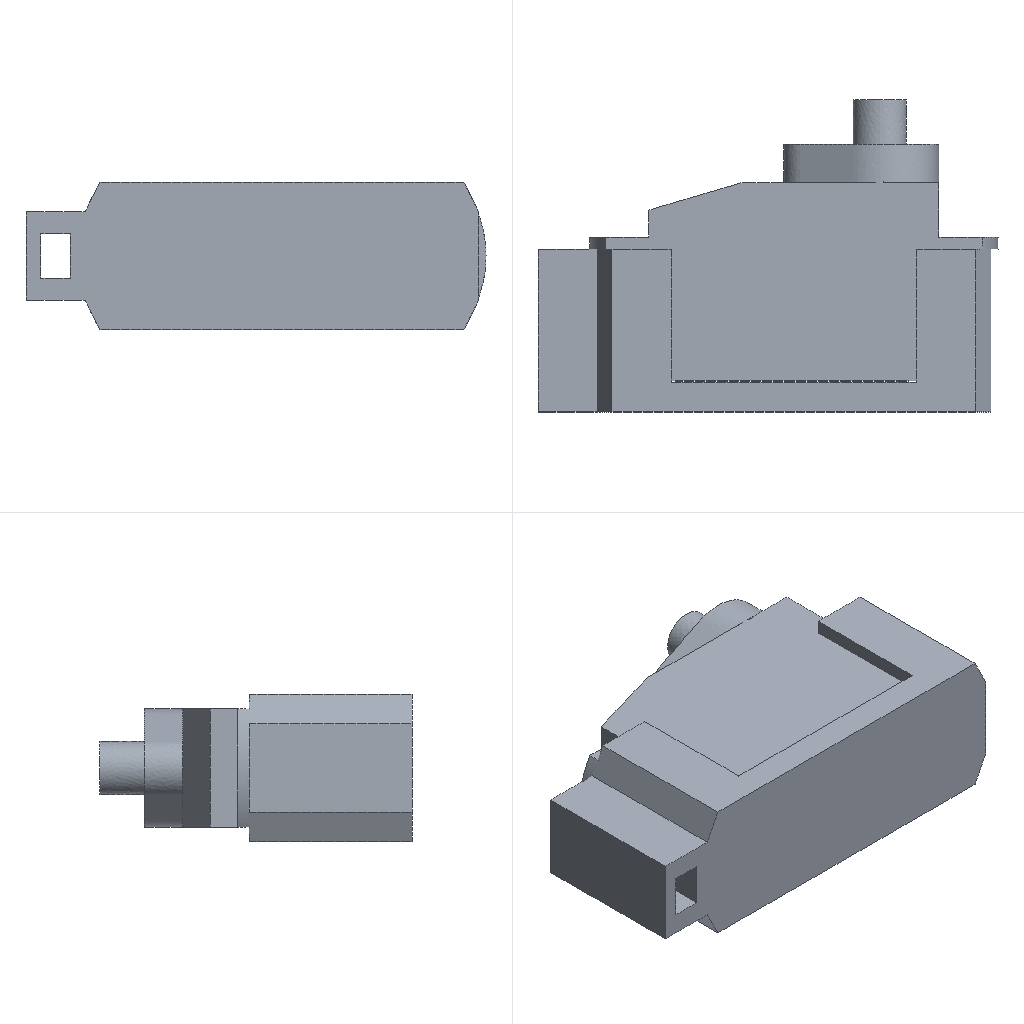Simulation study | ansys workbench
Ansys APDL input file, long lists of numbers shortened:
/batch
/config,noeldb,1     ! force off writing results to database
*get,_wallstrt,active,,time,wall
! ANSYS input file written by Workbench version 2022 R1
! File used for geometry attach: F:\ansys（分析文件汇总)\连杆和曲柄有限元分析\连杆1.STEP
/title,1--__ (D5)
! ****** Begin Custom Load Command Snippet ******
/COM, ACT Extensions:
/COM,     LSDYNA, 2021.1
/COM,
! ****** End   Custom Load Command Snippet ******
*DIM,_wb_ProjectScratch_dir,string,248
_wb_ProjectScratch_dir(1) = 'F:\ansys（分析文件汇总)\连杆和曲柄有限元分析\_ProjectScratch\Scr994B\'
*DIM,_wb_SolverFiles_dir,string,248
_wb_SolverFiles_dir(1) = 'F:\ansys（分析文件汇总)\连杆和曲柄有限元分析\1_files\dp0\SYS-1\MECH\'
*DIM,_wb_userfiles_dir,string,248
_wb_userfiles_dir(1) = 'F:\ansys（分析文件汇总)\连杆和曲柄有限元分析\1_files\user_files\'
/com,--- Data in consistent NMM units. See Solving Units in the help system for more information.
/units,MPA
/nopr
/wb,file,start              !  signify a WB generated input file
/prep7
! Turn off shape checking because checks already performed inside WB mesher.
! See help system for more information.
SHPP,OFF,,NOWARN
/nolist
etcon,set             ! allow ANSYS to choose best KEYOP's for 180x elements, resets any applicable keyopt to MAPDL defaults
/com,*********** Nodes for the whole assembly ***********
nblock,3,,1399
(1i9,3e20.9e3)
        1     1.020043493E+01     7.196480083E-01     5.000000000E-01
! (1271 more lines like these left out)
-1
/wb,elem,start            !  set before creation of elements
/com,*********** Elements for Body 1 "__1-FreeParts|____-____1" ***********
et,1,186
keyo,1,2,1          ! set full integration on SOLID186
eblock,19,solid,,190
(19i9)
        1        1        1        1        0        0        0        0       20        0        1        8      268       32       14      123      267       99      117
! (379 more lines like these left out)
-1
/wb,elem,end               !  done creating elements
/com,*********** Send User Defined Coordinate System(s) ***********
csys,0
toffst,273.15,  ! Temperature offset from absolute zero
/com,*********** Set Reference Temperature ***********
tref,22.
/wb,mat,start              !  starting to send materials
/com,*********** Send Materials ***********
Temperature = 'TEMP' ! Temperature
MP,DENS,1,1.05e-09,	! tonne mm^-3
MP,ALPX,1,1.2e-05,	! C^-1
MP,C,1,434000000,	! mm^2 s^-2 C^-1
MP,KXX,1,60.5,	! tonne mm s^-3 C^-1
MP,RSVX,1,0.00017,	! ohm mm
MP,EX,1,2300,	! tonne s^-2 mm^-1
MP,NUXY,1,0.39,
MP,MURX,1,10000,
/wb,mat,end                !  done sending materials
!************************* Model Summary ********************
!__1-FreeParts|____-____1,	ABS,	matid,	1
!************************* End Model Summary ********************
! get the diagonal of the bounding box. Needed later for other things
*get,_xmin,node,,mnloc,x
*get,_ymin,node,,mnloc,y
*get,_zmin,node,,mnloc,z
*get,_xmax,node,,mxloc,x
*get,_ymax,node,,mxloc,y
*get,_zmax,node,,mxloc,z
_ASMDIAG=(_xmax-_xmin)*(_xmax-_xmin)+(_ymax-_ymin)*(_ymax-_ymin)+(_zmax-_zmin)*(_zmax-_zmin)
_ASMDIAG=SQRT(_ASMDIAG)
/wb,contact,start          !  starting to send contact
/wb,contact,end            !  done creating contacts
/golist
/wb,load,start             !  starting to send loads
/com,*********** Fixed Supports ***********
CMBLOCK,_FIXEDSU,NODE,       96
(8i10)
       196       197       198       199       246       247       248       249
! (11 more lines like these left out)
cmsel,s,_FIXEDSU
d,all,all
nsel,all
/com,*********** Define Rotational Velocity ***********
cglo,0.,0.,0.
/gst,on,on
fini
*get,_numnode,node,0,count
*get,_numelem,elem,0,count
*get, _MAXELEMNUM, elem, 0, NUM, MAX
*get, _MAXNODENUM, node, 0, NUM, MAX
*get, _MAXELEMTYPE, etyp, 0, NUM, MAX
*get, _MAXREALCONST, real, 0, NUM, MAX
/go
/wb,load,end               !  done creating loads
/com,--- Number of total nodes = %_numnode%
/com,--- Number of contact elements = 0
/com,--- Number of spring elements = 0
/com,--- Number of bearing elements = 0
/com,--- Number of solid elements = 190
/com,--- Number of condensed parts = 0
/com,--- Number of total elements = %_numelem%
*get,_wallbsol,active,,time,wall
/com,****************************************************************************
/com,*************************    SOLUTION       ********************************
/com,****************************************************************************
/solu
antype,4                   ! transient analysis
nlgeom,on                  ! Turn on Large Deformation Effects
kbc,1                      ! stepped BC's
_thickRatio=  0     ! Ratio of thick parts in the model
eqsl,sparse,,,,,1
cntr,print,1               ! print out contact info and also make no initial contact an error
dmpoption,emat,no             ! Don't combine emat file for DANSYS
dmpoption,esav,no             ! Don't combine esav file for DANSYS
trnopt,full,,,,,hht        ! HHT time integration method
tintp, mosp			! Choose transient integration settings for moderate speed application
nldiag,cont,iter           ! print out contact info each equilibrium iteration
rescontrol,define,last,last,,dele	   ! Program Controlled
/com,****************************************************
/com,******************* SOLVE FOR LS 1 OF 1 ****************
cgom,10.,0.,0.
/nopr
/gopr
autots,on                   ! User turned on automatic time stepping
deltim,1,1,1,OFF
time,1.
timint,on                  ! Turn on time integration effects
outres,erase
outres,all,none
outres,nsol,all,
outres,rsol,all
outres,eangl,all
outres,etmp,all
outres,veng,all
outres,strs,all,
outres,epel,all,
outres,eppl,all,
outres,cont,all,
outres,v,all,
outres,a,all,
! *********** WB SOLVE COMMAND ***********
! check interactive state
*get,ANSINTER_,active,,int
*if,ANSINTER_,ne,0,then
/eof
*endif
solve
/com *************** Write FE CONNECTORS *********
CEWRITE,file,ce,,INTE
/com,****************************************************
/com,*************** FINISHED SOLVE FOR LS 1 *************
*get,_wallasol,active,,time,wall
/nopr
*get,_numnode,node,0,count
*get,_numelem,elem,0,count
*get, _MAXELEMNUM, elem, 0, NUM, MAX
*get, _MAXNODENUM, node, 0, NUM, MAX,,,INTERNAL
*get, _MAXELEMTYPE, etyp, 0, NUM, MAX
*get, _MAXREALCONST, real, 0, NUM, MAX
/gopr
/post1
xmlo,ENCODING,ISO-8859-1
xmlo,parm
/xml,parm,xml
fini
/gopr
*get,_walldone,active,,time,wall
_preptime=(_wallbsol-_wallstrt)*3600
_solvtime=(_wallasol-_wallbsol)*3600
_posttime=(_walldone-_wallasol)*3600
_totaltim=(_walldone-_wallstrt)*3600
*get,_dlbratio,active,0,solu,dlbr
*get,_combtime,active,0,solu,comb
*get,_ssmode,active,0,solu,ssmm
*get,_ndofs,active,0,solu,ndof
*get,_sol_end_time,active,0,set,time
*if,_sol_end_time,eq,1.,then
/fclean				!clean distributed files
*endif
/com,--- Total number of nodes = %_numnode%
/com,--- Total number of elements = %_numelem%
/com,--- Element load balance ratio = %_dlbratio%
/com,--- Time to combine distributed files = %_combtime%
/com,--- Sparse memory mode = %_ssmode%
/com,--- Number of DOF = %_ndofs%
/wb,file,end               ! done with WB generated input